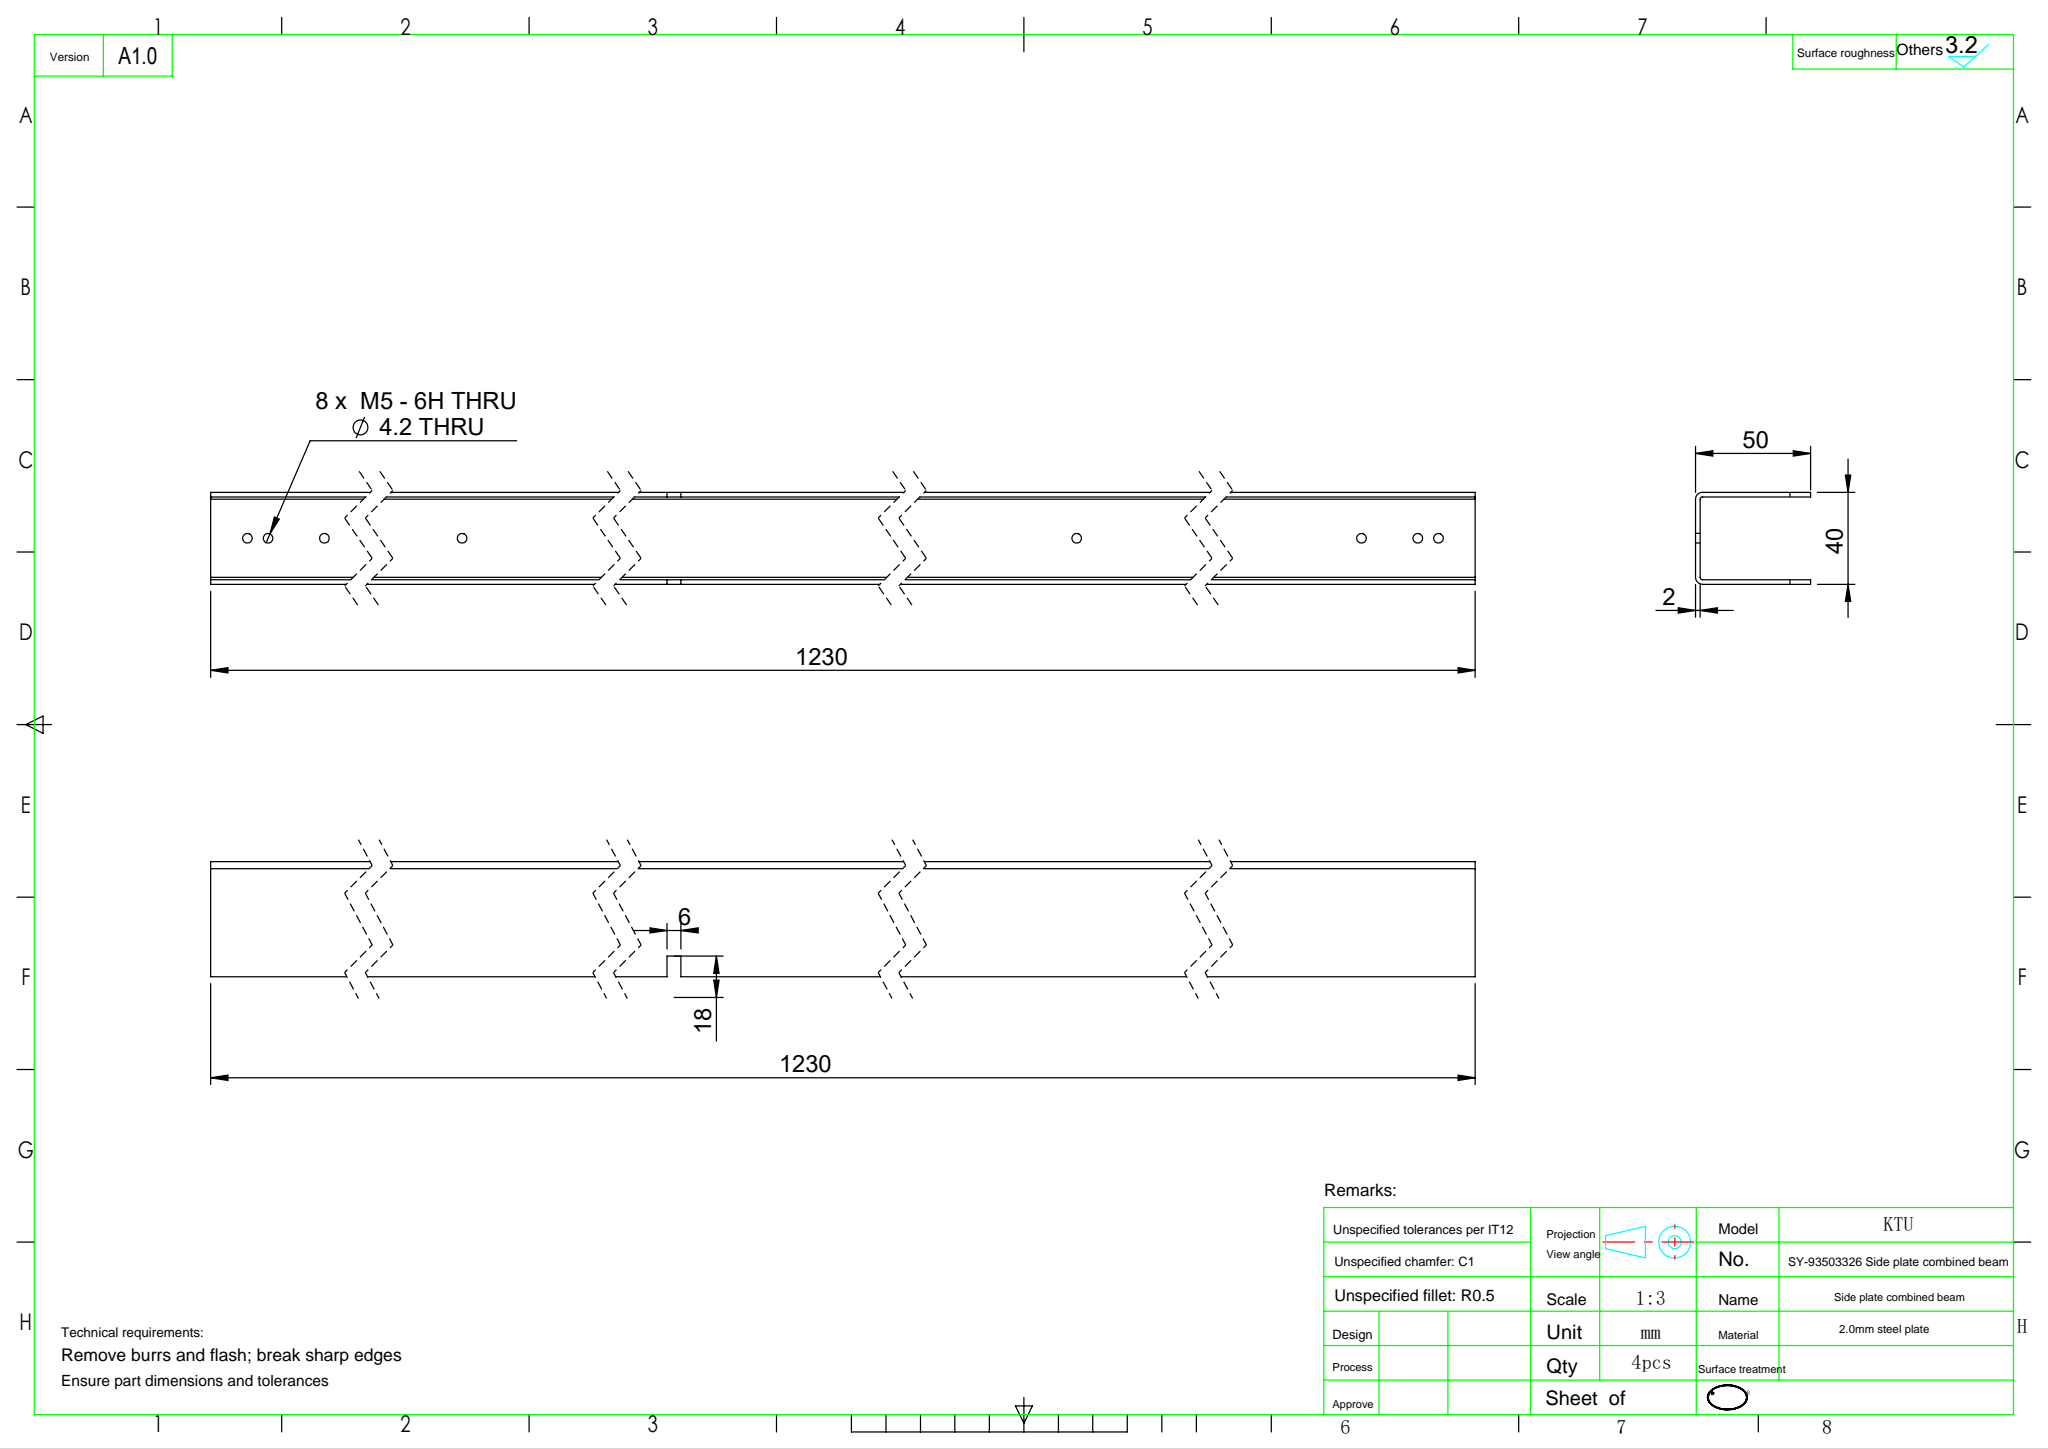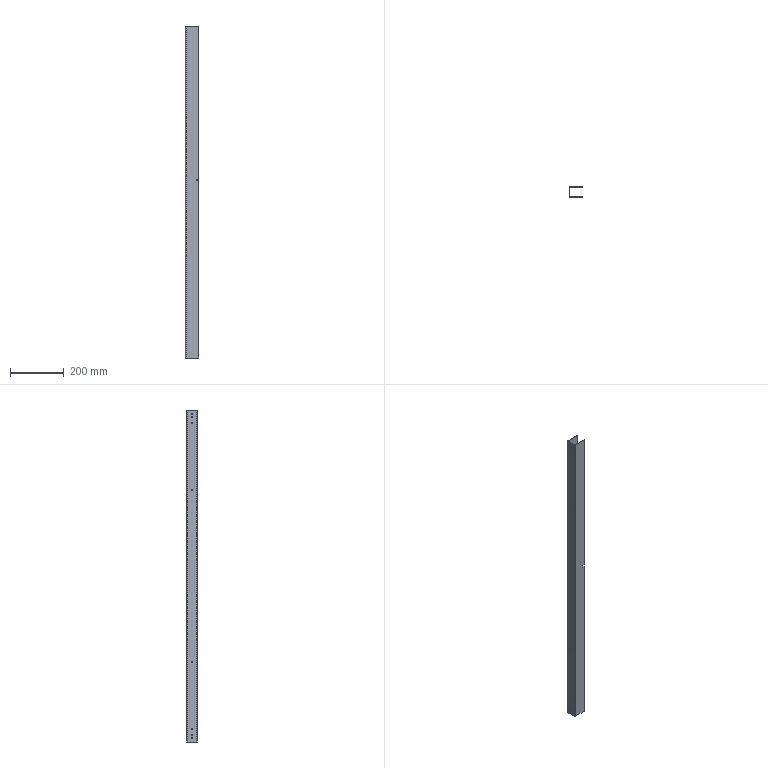Part | SolidWorks | features Cut 1, ExtruThin 1, HoleWzd 1 | 1 solid | 38 faces | box 50 x 40 x 1230 mm | volume 329899 mm3 | cylinder 20 | plane 18 | commonest cylinder face diameters 4.2 x16 2 x2 6 x2